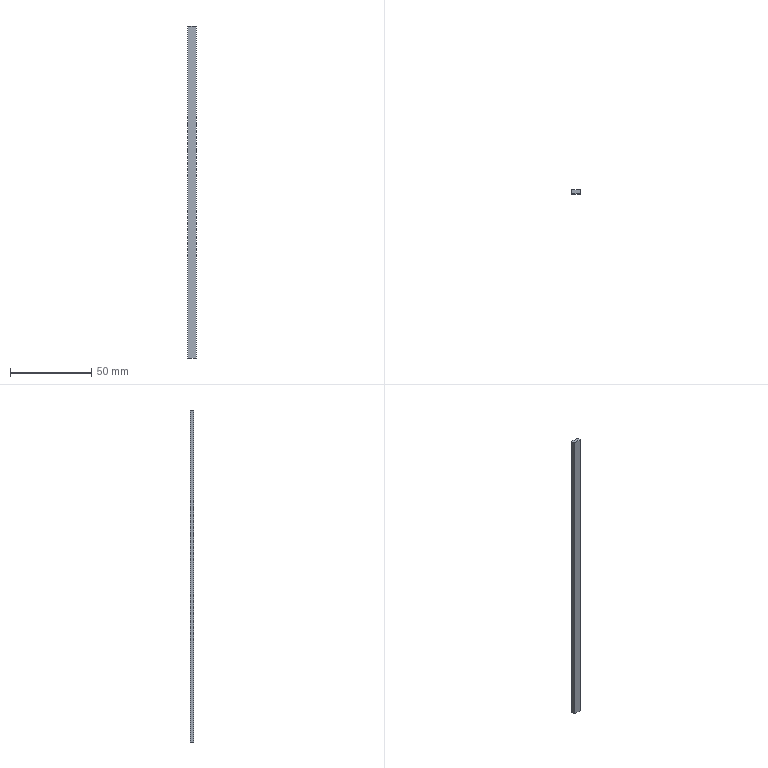Part | SolidWorks | features FlatPattern 1, SMBaseFlange 1, SheetMetal 1 | 1 solid | 6 faces | box 5 x 2.3 x 204.8 mm | volume 2355 mm3 | plane 6
STEP:
#1=CARTESIAN_POINT('',(2.5,0.,102.4));
#2=VERTEX_POINT('',#1);
#3=CARTESIAN_POINT('',(2.5,0.,-102.4));
#4=VERTEX_POINT('',#3);
#5=CARTESIAN_POINT('',(2.5,0.,-102.4));
#6=DIRECTION('',(0.,0.,-1.));
#7=VECTOR('',#6,1000.);
#8=LINE('',#5,#7);
#9=EDGE_CURVE('',#2,#4,#8,.T.);
#10=ORIENTED_EDGE('',*,*,#9,.F.);
#11=CARTESIAN_POINT('',(2.5,-2.3,102.4));
#12=VERTEX_POINT('',#11);
#13=CARTESIAN_POINT('',(2.5,-2.3,102.4));
#14=DIRECTION('',(0.,1.,0.));
#15=VECTOR('',#14,1000.);
#16=LINE('',#13,#15);
#17=EDGE_CURVE('',#12,#2,#16,.T.);
#18=ORIENTED_EDGE('',*,*,#17,.F.);
#19=CARTESIAN_POINT('',(2.5,-2.3,-102.4));
#20=VERTEX_POINT('',#19);
#21=CARTESIAN_POINT('',(2.5,-2.3,-102.4));
#22=DIRECTION('',(0.,0.,-1.));
#23=VECTOR('',#22,1000.);
#24=LINE('',#21,#23);
#25=EDGE_CURVE('',#12,#20,#24,.T.);
#26=ORIENTED_EDGE('',*,*,#25,.T.);
#27=CARTESIAN_POINT('',(2.5,-2.3,-102.4));
#28=DIRECTION('',(0.,1.,0.));
#29=VECTOR('',#28,1000.);
#30=LINE('',#27,#29);
#31=EDGE_CURVE('',#20,#4,#30,.T.);
#32=ORIENTED_EDGE('',*,*,#31,.T.);
#33=EDGE_LOOP('',(#10,#18,#26,#32));
#34=FACE_OUTER_BOUND('',#33,.T.);
#35=CARTESIAN_POINT('',(2.5,-2.3,-102.4));
#36=DIRECTION('',(1.,0.,0.));
#37=DIRECTION('',(0.,0.,-1.));
#38=AXIS2_PLACEMENT_3D('',#35,#36,#37);
#39=PLANE('',#38);
#40=ADVANCED_FACE('',(#34),#39,.T.);
#41=CARTESIAN_POINT('',(-2.5,0.,102.4));
#42=VERTEX_POINT('',#41);
#43=CARTESIAN_POINT('',(-2.5,0.,102.4));
#44=DIRECTION('',(1.,0.,0.));
#45=VECTOR('',#44,1000.);
#46=LINE('',#43,#45);
#47=EDGE_CURVE('',#42,#2,#46,.T.);
#48=ORIENTED_EDGE('',*,*,#47,.F.);
#49=CARTESIAN_POINT('',(-2.5,-2.3,102.4));
#50=VERTEX_POINT('',#49);
#51=CARTESIAN_POINT('',(-2.5,-2.3,102.4));
#52=DIRECTION('',(0.,1.,0.));
#53=VECTOR('',#52,1000.);
#54=LINE('',#51,#53);
#55=EDGE_CURVE('',#50,#42,#54,.T.);
#56=ORIENTED_EDGE('',*,*,#55,.F.);
#57=CARTESIAN_POINT('',(-2.5,-2.3,102.4));
#58=DIRECTION('',(1.,0.,0.));
#59=VECTOR('',#58,1000.);
#60=LINE('',#57,#59);
#61=EDGE_CURVE('',#50,#12,#60,.T.);
#62=ORIENTED_EDGE('',*,*,#61,.T.);
#63=ORIENTED_EDGE('',*,*,#17,.T.);
#64=EDGE_LOOP('',(#48,#56,#62,#63));
#65=FACE_OUTER_BOUND('',#64,.T.);
#66=CARTESIAN_POINT('',(-2.5,-2.3,102.4));
#67=DIRECTION('',(0.,0.,1.));
#68=DIRECTION('',(1.,0.,0.));
#69=AXIS2_PLACEMENT_3D('',#66,#67,#68);
#70=PLANE('',#69);
#71=ADVANCED_FACE('',(#65),#70,.T.);
#72=CARTESIAN_POINT('',(-2.5,0.,-102.4));
#73=VERTEX_POINT('',#72);
#74=CARTESIAN_POINT('',(-2.5,0.,-102.4));
#75=DIRECTION('',(0.,0.,1.));
#76=VECTOR('',#75,1000.);
#77=LINE('',#74,#76);
#78=EDGE_CURVE('',#73,#42,#77,.T.);
#79=ORIENTED_EDGE('',*,*,#78,.F.);
#80=CARTESIAN_POINT('',(-2.5,-2.3,-102.4));
#81=VERTEX_POINT('',#80);
#82=CARTESIAN_POINT('',(-2.5,-2.3,-102.4));
#83=DIRECTION('',(0.,1.,0.));
#84=VECTOR('',#83,1000.);
#85=LINE('',#82,#84);
#86=EDGE_CURVE('',#81,#73,#85,.T.);
#87=ORIENTED_EDGE('',*,*,#86,.F.);
#88=CARTESIAN_POINT('',(-2.5,-2.3,-102.4));
#89=DIRECTION('',(0.,0.,1.));
#90=VECTOR('',#89,1000.);
#91=LINE('',#88,#90);
#92=EDGE_CURVE('',#81,#50,#91,.T.);
#93=ORIENTED_EDGE('',*,*,#92,.T.);
#94=ORIENTED_EDGE('',*,*,#55,.T.);
#95=EDGE_LOOP('',(#79,#87,#93,#94));
#96=FACE_OUTER_BOUND('',#95,.T.);
#97=CARTESIAN_POINT('',(-2.5,-2.3,-102.4));
#98=DIRECTION('',(-1.,0.,0.));
#99=DIRECTION('',(0.,0.,1.));
#100=AXIS2_PLACEMENT_3D('',#97,#98,#99);
#101=PLANE('',#100);
#102=ADVANCED_FACE('',(#96),#101,.T.);
#103=CARTESIAN_POINT('',(-2.5,0.,-102.4));
#104=DIRECTION('',(-1.,0.,0.));
#105=VECTOR('',#104,1000.);
#106=LINE('',#103,#105);
#107=EDGE_CURVE('',#4,#73,#106,.T.);
#108=ORIENTED_EDGE('',*,*,#107,.F.);
#109=ORIENTED_EDGE('',*,*,#31,.F.);
#110=CARTESIAN_POINT('',(-2.5,-2.3,-102.4));
#111=DIRECTION('',(-1.,0.,0.));
#112=VECTOR('',#111,1000.);
#113=LINE('',#110,#112);
#114=EDGE_CURVE('',#20,#81,#113,.T.);
#115=ORIENTED_EDGE('',*,*,#114,.T.);
#116=ORIENTED_EDGE('',*,*,#86,.T.);
#117=EDGE_LOOP('',(#108,#109,#115,#116));
#118=FACE_OUTER_BOUND('',#117,.T.);
#119=CARTESIAN_POINT('',(-2.5,-2.3,-102.4));
#120=DIRECTION('',(0.,0.,-1.));
#121=DIRECTION('',(-1.,0.,0.));
#122=AXIS2_PLACEMENT_3D('',#119,#120,#121);
#123=PLANE('',#122);
#124=ADVANCED_FACE('',(#118),#123,.T.);
#125=ORIENTED_EDGE('',*,*,#25,.F.);
#126=ORIENTED_EDGE('',*,*,#61,.F.);
#127=ORIENTED_EDGE('',*,*,#92,.F.);
#128=ORIENTED_EDGE('',*,*,#114,.F.);
#129=EDGE_LOOP('',(#125,#126,#127,#128));
#130=FACE_OUTER_BOUND('',#129,.T.);
#131=CARTESIAN_POINT('',(0.,-2.3,0.));
#132=DIRECTION('',(0.,1.,0.));
#133=DIRECTION('',(0.,0.,1.));
#134=AXIS2_PLACEMENT_3D('',#131,#132,#133);
#135=PLANE('',#134);
#136=ADVANCED_FACE('',(#130),#135,.F.);
#137=ORIENTED_EDGE('',*,*,#9,.T.);
#138=ORIENTED_EDGE('',*,*,#107,.T.);
#139=ORIENTED_EDGE('',*,*,#78,.T.);
#140=ORIENTED_EDGE('',*,*,#47,.T.);
#141=EDGE_LOOP('',(#137,#138,#139,#140));
#142=FACE_OUTER_BOUND('',#141,.T.);
#143=CARTESIAN_POINT('',(0.,0.,0.));
#144=DIRECTION('',(0.,1.,0.));
#145=DIRECTION('',(0.,0.,1.));
#146=AXIS2_PLACEMENT_3D('',#143,#144,#145);
#147=PLANE('',#146);
#148=ADVANCED_FACE('',(#142),#147,.T.);
#149=CLOSED_SHELL('',(#40,#71,#102,#124,#136,#148));
#150=MANIFOLD_SOLID_BREP('',#149);
#151=CARTESIAN_POINT('',(0.,0.,0.));
#152=DIRECTION('',(0.,0.,1.));
#153=DIRECTION('',(1.,0.,0.));
#154=AXIS2_PLACEMENT_3D('',#151,#152,#153);
#155=(LENGTH_UNIT()NAMED_UNIT(*)SI_UNIT(.MILLI.,.METRE.));
#156=UNCERTAINTY_MEASURE_WITH_UNIT(LENGTH_MEASURE(0.00001),#155,'','');
#157=(NAMED_UNIT(*)PLANE_ANGLE_UNIT()SI_UNIT($,.RADIAN.));
#158=(NAMED_UNIT(*)SI_UNIT($,.STERADIAN.)SOLID_ANGLE_UNIT());
#159=(GEOMETRIC_REPRESENTATION_CONTEXT(3)GLOBAL_UNCERTAINTY_ASSIGNED_CONTEXT((#156))GLOBAL_UNIT_ASSIGNED_CONTEXT((#155,#157,#158))REPRESENTATION_CONTEXT('',''));
#160=ADVANCED_BREP_SHAPE_REPRESENTATION('',(#150,#154),#159);